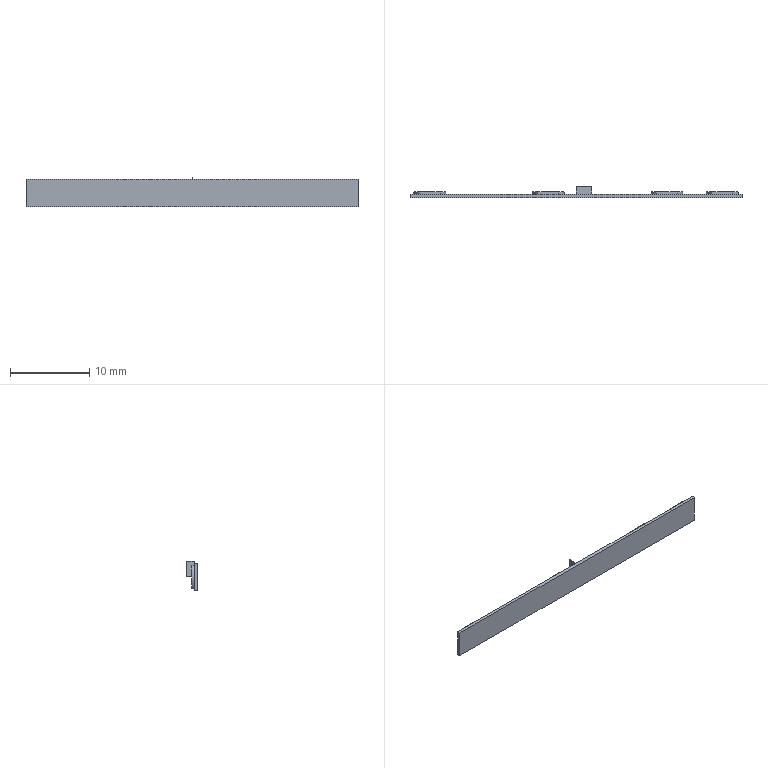Part | Creo | 1 solid | 28 faces | box 42 x 1.4 x 3.75 mm | volume 72.804 mm3 | plane 20 | cylinder 8 | commonest cylinder face diameters 4 x8